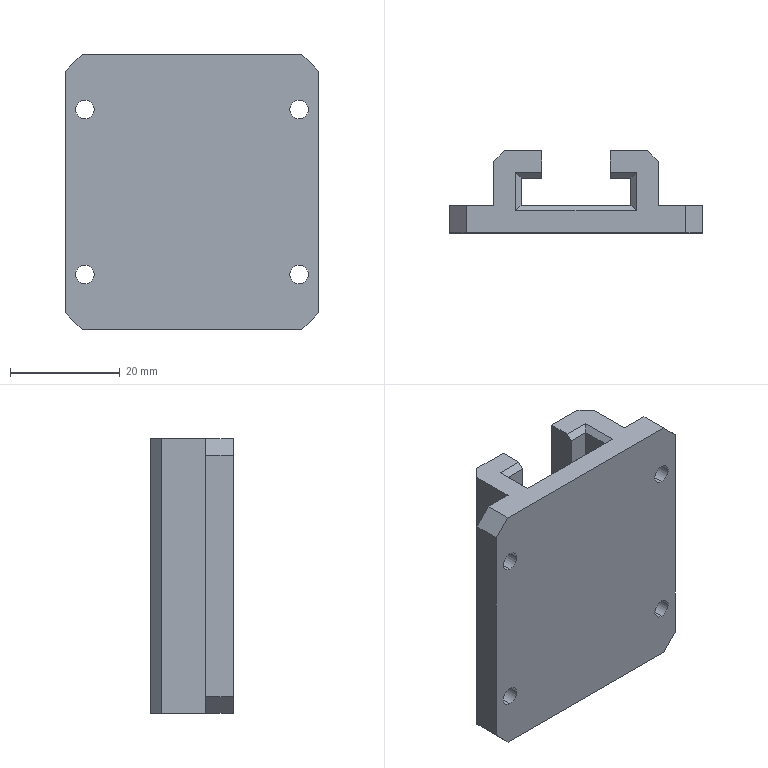Part | SolidWorks | features Chamfer 4, Extrusion 1, HoleWzd 1, ICE 1 | 1 solid | 42 faces | box 46 x 15 x 50 mm | volume 17863 mm3 | plane 34 | cylinder 8 | commonest cylinder face diameters 3.4 x8
STEP:
#1=CARTESIAN_POINT('',(-19.5,0.,8.3));
#2=VERTEX_POINT('',#1);
#3=CARTESIAN_POINT('',(-19.5,0.,11.7));
#4=VERTEX_POINT('',#3);
#5=CARTESIAN_POINT('',(-19.5,0.,10.));
#6=DIRECTION('',(0.,1.,0.));
#7=DIRECTION('',(0.,0.,1.));
#8=AXIS2_PLACEMENT_3D('',#5,#6,#7);
#9=CIRCLE('',#8,1.7);
#10=EDGE_CURVE('',#2,#4,#9,.T.);
#11=ORIENTED_EDGE('',*,*,#10,.F.);
#12=CARTESIAN_POINT('',(-19.5,5.,8.3));
#13=VERTEX_POINT('',#12);
#14=CARTESIAN_POINT('',(-19.5,5.,8.3));
#15=DIRECTION('',(0.,1.,0.));
#16=VECTOR('',#15,1000.);
#17=LINE('',#14,#16);
#18=EDGE_CURVE('',#2,#13,#17,.T.);
#19=ORIENTED_EDGE('',*,*,#18,.T.);
#20=CARTESIAN_POINT('',(-19.5,5.,11.7));
#21=VERTEX_POINT('',#20);
#22=CARTESIAN_POINT('',(-19.5,5.,10.));
#23=DIRECTION('',(0.,1.,0.));
#24=DIRECTION('',(0.,0.,1.));
#25=AXIS2_PLACEMENT_3D('',#22,#23,#24);
#26=CIRCLE('',#25,1.7);
#27=EDGE_CURVE('',#13,#21,#26,.T.);
#28=ORIENTED_EDGE('',*,*,#27,.T.);
#29=CARTESIAN_POINT('',(-19.5,5.,11.7));
#30=DIRECTION('',(0.,1.,0.));
#31=VECTOR('',#30,1000.);
#32=LINE('',#29,#31);
#33=EDGE_CURVE('',#4,#21,#32,.T.);
#34=ORIENTED_EDGE('',*,*,#33,.F.);
#35=EDGE_LOOP('',(#11,#19,#28,#34));
#36=FACE_OUTER_BOUND('',#35,.T.);
#37=CARTESIAN_POINT('',(-19.5,5.,10.));
#38=DIRECTION('',(0.,1.,0.));
#39=DIRECTION('',(0.,0.,1.));
#40=AXIS2_PLACEMENT_3D('',#37,#38,#39);
#41=CYLINDRICAL_SURFACE('',#40,1.7);
#42=ADVANCED_FACE('',(#36),#41,.F.);
#43=CARTESIAN_POINT('',(-19.5,0.,38.3));
#44=VERTEX_POINT('',#43);
#45=CARTESIAN_POINT('',(-19.5,0.,41.7));
#46=VERTEX_POINT('',#45);
#47=CARTESIAN_POINT('',(-19.5,0.,40.));
#48=DIRECTION('',(0.,1.,0.));
#49=DIRECTION('',(0.,0.,1.));
#50=AXIS2_PLACEMENT_3D('',#47,#48,#49);
#51=CIRCLE('',#50,1.7);
#52=EDGE_CURVE('',#44,#46,#51,.T.);
#53=ORIENTED_EDGE('',*,*,#52,.F.);
#54=CARTESIAN_POINT('',(-19.5,5.,38.3));
#55=VERTEX_POINT('',#54);
#56=CARTESIAN_POINT('',(-19.5,5.,38.3));
#57=DIRECTION('',(0.,1.,0.));
#58=VECTOR('',#57,1000.);
#59=LINE('',#56,#58);
#60=EDGE_CURVE('',#44,#55,#59,.T.);
#61=ORIENTED_EDGE('',*,*,#60,.T.);
#62=CARTESIAN_POINT('',(-19.5,5.,41.7));
#63=VERTEX_POINT('',#62);
#64=CARTESIAN_POINT('',(-19.5,5.,40.));
#65=DIRECTION('',(0.,1.,0.));
#66=DIRECTION('',(0.,0.,1.));
#67=AXIS2_PLACEMENT_3D('',#64,#65,#66);
#68=CIRCLE('',#67,1.7);
#69=EDGE_CURVE('',#55,#63,#68,.T.);
#70=ORIENTED_EDGE('',*,*,#69,.T.);
#71=CARTESIAN_POINT('',(-19.5,5.,41.7));
#72=DIRECTION('',(0.,1.,0.));
#73=VECTOR('',#72,1000.);
#74=LINE('',#71,#73);
#75=EDGE_CURVE('',#46,#63,#74,.T.);
#76=ORIENTED_EDGE('',*,*,#75,.F.);
#77=EDGE_LOOP('',(#53,#61,#70,#76));
#78=FACE_OUTER_BOUND('',#77,.T.);
#79=CARTESIAN_POINT('',(-19.5,5.,40.));
#80=DIRECTION('',(0.,1.,0.));
#81=DIRECTION('',(0.,0.,1.));
#82=AXIS2_PLACEMENT_3D('',#79,#80,#81);
#83=CYLINDRICAL_SURFACE('',#82,1.7);
#84=ADVANCED_FACE('',(#78),#83,.F.);
#85=CARTESIAN_POINT('',(19.5,0.,38.3));
#86=VERTEX_POINT('',#85);
#87=CARTESIAN_POINT('',(19.5,0.,41.7));
#88=VERTEX_POINT('',#87);
#89=CARTESIAN_POINT('',(19.5,0.,40.));
#90=DIRECTION('',(0.,1.,0.));
#91=DIRECTION('',(0.,0.,1.));
#92=AXIS2_PLACEMENT_3D('',#89,#90,#91);
#93=CIRCLE('',#92,1.7);
#94=EDGE_CURVE('',#86,#88,#93,.T.);
#95=ORIENTED_EDGE('',*,*,#94,.F.);
#96=CARTESIAN_POINT('',(19.5,5.,38.3));
#97=VERTEX_POINT('',#96);
#98=CARTESIAN_POINT('',(19.5,5.,38.3));
#99=DIRECTION('',(0.,1.,0.));
#100=VECTOR('',#99,1000.);
#101=LINE('',#98,#100);
#102=EDGE_CURVE('',#86,#97,#101,.T.);
#103=ORIENTED_EDGE('',*,*,#102,.T.);
#104=CARTESIAN_POINT('',(19.5,5.,41.7));
#105=VERTEX_POINT('',#104);
#106=CARTESIAN_POINT('',(19.5,5.,40.));
#107=DIRECTION('',(0.,1.,0.));
#108=DIRECTION('',(0.,0.,1.));
#109=AXIS2_PLACEMENT_3D('',#106,#107,#108);
#110=CIRCLE('',#109,1.7);
#111=EDGE_CURVE('',#97,#105,#110,.T.);
#112=ORIENTED_EDGE('',*,*,#111,.T.);
#113=CARTESIAN_POINT('',(19.5,5.,41.7));
#114=DIRECTION('',(0.,1.,0.));
#115=VECTOR('',#114,1000.);
#116=LINE('',#113,#115);
#117=EDGE_CURVE('',#88,#105,#116,.T.);
#118=ORIENTED_EDGE('',*,*,#117,.F.);
#119=EDGE_LOOP('',(#95,#103,#112,#118));
#120=FACE_OUTER_BOUND('',#119,.T.);
#121=CARTESIAN_POINT('',(19.5,5.,40.));
#122=DIRECTION('',(0.,1.,0.));
#123=DIRECTION('',(0.,0.,1.));
#124=AXIS2_PLACEMENT_3D('',#121,#122,#123);
#125=CYLINDRICAL_SURFACE('',#124,1.7);
#126=ADVANCED_FACE('',(#120),#125,.F.);
#127=CARTESIAN_POINT('',(19.5,0.,8.3));
#128=VERTEX_POINT('',#127);
#129=CARTESIAN_POINT('',(19.5,0.,11.7));
#130=VERTEX_POINT('',#129);
#131=CARTESIAN_POINT('',(19.5,0.,10.));
#132=DIRECTION('',(0.,1.,0.));
#133=DIRECTION('',(0.,0.,1.));
#134=AXIS2_PLACEMENT_3D('',#131,#132,#133);
#135=CIRCLE('',#134,1.7);
#136=EDGE_CURVE('',#128,#130,#135,.T.);
#137=ORIENTED_EDGE('',*,*,#136,.F.);
#138=CARTESIAN_POINT('',(19.5,5.,8.3));
#139=VERTEX_POINT('',#138);
#140=CARTESIAN_POINT('',(19.5,5.,8.3));
#141=DIRECTION('',(0.,1.,0.));
#142=VECTOR('',#141,1000.);
#143=LINE('',#140,#142);
#144=EDGE_CURVE('',#128,#139,#143,.T.);
#145=ORIENTED_EDGE('',*,*,#144,.T.);
#146=CARTESIAN_POINT('',(19.5,5.,11.7));
#147=VERTEX_POINT('',#146);
#148=CARTESIAN_POINT('',(19.5,5.,10.));
#149=DIRECTION('',(0.,1.,0.));
#150=DIRECTION('',(0.,0.,1.));
#151=AXIS2_PLACEMENT_3D('',#148,#149,#150);
#152=CIRCLE('',#151,1.7);
#153=EDGE_CURVE('',#139,#147,#152,.T.);
#154=ORIENTED_EDGE('',*,*,#153,.T.);
#155=CARTESIAN_POINT('',(19.5,5.,11.7));
#156=DIRECTION('',(0.,1.,0.));
#157=VECTOR('',#156,1000.);
#158=LINE('',#155,#157);
#159=EDGE_CURVE('',#130,#147,#158,.T.);
#160=ORIENTED_EDGE('',*,*,#159,.F.);
#161=EDGE_LOOP('',(#137,#145,#154,#160));
#162=FACE_OUTER_BOUND('',#161,.T.);
#163=CARTESIAN_POINT('',(19.5,5.,10.));
#164=DIRECTION('',(0.,1.,0.));
#165=DIRECTION('',(0.,0.,1.));
#166=AXIS2_PLACEMENT_3D('',#163,#164,#165);
#167=CYLINDRICAL_SURFACE('',#166,1.7);
#168=ADVANCED_FACE('',(#162),#167,.F.);
#169=CARTESIAN_POINT('',(15.,5.,0.));
#170=VERTEX_POINT('',#169);
#171=CARTESIAN_POINT('',(15.,13.,0.));
#172=VERTEX_POINT('',#171);
#173=CARTESIAN_POINT('',(15.,0.,0.));
#174=DIRECTION('',(0.,1.,0.));
#175=VECTOR('',#174,1000.);
#176=LINE('',#173,#175);
#177=EDGE_CURVE('',#170,#172,#176,.T.);
#178=ORIENTED_EDGE('',*,*,#177,.T.);
#179=CARTESIAN_POINT('',(15.,13.,50.));
#180=VERTEX_POINT('',#179);
#181=CARTESIAN_POINT('',(15.,13.,50.));
#182=DIRECTION('',(0.,0.,1.));
#183=VECTOR('',#182,1000.);
#184=LINE('',#181,#183);
#185=EDGE_CURVE('',#172,#180,#184,.T.);
#186=ORIENTED_EDGE('',*,*,#185,.T.);
#187=CARTESIAN_POINT('',(15.,5.,50.));
#188=VERTEX_POINT('',#187);
#189=CARTESIAN_POINT('',(15.,0.,50.));
#190=DIRECTION('',(0.,1.,0.));
#191=VECTOR('',#190,1000.);
#192=LINE('',#189,#191);
#193=EDGE_CURVE('',#188,#180,#192,.T.);
#194=ORIENTED_EDGE('',*,*,#193,.F.);
#195=CARTESIAN_POINT('',(15.,5.,-9.434));
#196=DIRECTION('',(0.,0.,1.));
#197=VECTOR('',#196,1000.);
#198=LINE('',#195,#197);
#199=EDGE_CURVE('',#170,#188,#198,.T.);
#200=ORIENTED_EDGE('',*,*,#199,.F.);
#201=EDGE_LOOP('',(#178,#186,#194,#200));
#202=FACE_OUTER_BOUND('',#201,.T.);
#203=CARTESIAN_POINT('',(15.,0.,50.));
#204=DIRECTION('',(-1.,0.,0.));
#205=DIRECTION('',(0.,0.,1.));
#206=AXIS2_PLACEMENT_3D('',#203,#204,#205);
#207=PLANE('',#206);
#208=ADVANCED_FACE('',(#202),#207,.F.);
#209=CARTESIAN_POINT('',(-15.,13.,50.));
#210=VERTEX_POINT('',#209);
#211=CARTESIAN_POINT('',(-15.,5.,50.));
#212=VERTEX_POINT('',#211);
#213=CARTESIAN_POINT('',(-15.,0.,50.));
#214=DIRECTION('',(0.,-1.,0.));
#215=VECTOR('',#214,1000.);
#216=LINE('',#213,#215);
#217=EDGE_CURVE('',#210,#212,#216,.T.);
#218=ORIENTED_EDGE('',*,*,#217,.F.);
#219=CARTESIAN_POINT('',(-15.,13.,0.));
#220=VERTEX_POINT('',#219);
#221=CARTESIAN_POINT('',(-15.,13.,50.));
#222=DIRECTION('',(0.,0.,-1.));
#223=VECTOR('',#222,1000.);
#224=LINE('',#221,#223);
#225=EDGE_CURVE('',#210,#220,#224,.T.);
#226=ORIENTED_EDGE('',*,*,#225,.T.);
#227=CARTESIAN_POINT('',(-15.,5.,0.));
#228=VERTEX_POINT('',#227);
#229=CARTESIAN_POINT('',(-15.,0.,0.));
#230=DIRECTION('',(0.,-1.,0.));
#231=VECTOR('',#230,1000.);
#232=LINE('',#229,#231);
#233=EDGE_CURVE('',#220,#228,#232,.T.);
#234=ORIENTED_EDGE('',*,*,#233,.T.);
#235=CARTESIAN_POINT('',(-15.,5.,-9.434));
#236=DIRECTION('',(0.,0.,1.));
#237=VECTOR('',#236,1000.);
#238=LINE('',#235,#237);
#239=EDGE_CURVE('',#228,#212,#238,.T.);
#240=ORIENTED_EDGE('',*,*,#239,.T.);
#241=EDGE_LOOP('',(#218,#226,#234,#240));
#242=FACE_OUTER_BOUND('',#241,.T.);
#243=CARTESIAN_POINT('',(-15.,0.,50.));
#244=DIRECTION('',(1.,0.,0.));
#245=DIRECTION('',(0.,0.,-1.));
#246=AXIS2_PLACEMENT_3D('',#243,#244,#245);
#247=PLANE('',#246);
#248=ADVANCED_FACE('',(#242),#247,.F.);
#249=CARTESIAN_POINT('',(-19.5,0.,10.));
#250=DIRECTION('',(0.,1.,0.));
#251=DIRECTION('',(0.,0.,1.));
#252=AXIS2_PLACEMENT_3D('',#249,#250,#251);
#253=CIRCLE('',#252,1.7);
#254=EDGE_CURVE('',#4,#2,#253,.T.);
#255=ORIENTED_EDGE('',*,*,#254,.T.);
#256=ORIENTED_EDGE('',*,*,#10,.T.);
#257=EDGE_LOOP('',(#255,#256));
#258=FACE_BOUND('',#257,.T.);
#259=CARTESIAN_POINT('',(-19.5,0.,40.));
#260=DIRECTION('',(0.,1.,0.));
#261=DIRECTION('',(0.,0.,1.));
#262=AXIS2_PLACEMENT_3D('',#259,#260,#261);
#263=CIRCLE('',#262,1.7);
#264=EDGE_CURVE('',#46,#44,#263,.T.);
#265=ORIENTED_EDGE('',*,*,#264,.T.);
#266=ORIENTED_EDGE('',*,*,#52,.T.);
#267=EDGE_LOOP('',(#265,#266));
#268=FACE_BOUND('',#267,.T.);
#269=CARTESIAN_POINT('',(19.5,0.,40.));
#270=DIRECTION('',(0.,1.,0.));
#271=DIRECTION('',(0.,0.,1.));
#272=AXIS2_PLACEMENT_3D('',#269,#270,#271);
#273=CIRCLE('',#272,1.7);
#274=EDGE_CURVE('',#88,#86,#273,.T.);
#275=ORIENTED_EDGE('',*,*,#274,.T.);
#276=ORIENTED_EDGE('',*,*,#94,.T.);
#277=EDGE_LOOP('',(#275,#276));
#278=FACE_BOUND('',#277,.T.);
#279=CARTESIAN_POINT('',(19.5,0.,10.));
#280=DIRECTION('',(0.,1.,0.));
#281=DIRECTION('',(0.,0.,1.));
#282=AXIS2_PLACEMENT_3D('',#279,#280,#281);
#283=CIRCLE('',#282,1.7);
#284=EDGE_CURVE('',#130,#128,#283,.T.);
#285=ORIENTED_EDGE('',*,*,#284,.T.);
#286=ORIENTED_EDGE('',*,*,#136,.T.);
#287=EDGE_LOOP('',(#285,#286));
#288=FACE_BOUND('',#287,.T.);
#289=CARTESIAN_POINT('',(-23.,0.,3.));
#290=VERTEX_POINT('',#289);
#291=CARTESIAN_POINT('',(-23.,0.,47.));
#292=VERTEX_POINT('',#291);
#293=CARTESIAN_POINT('',(-23.,0.,-9.434));
#294=DIRECTION('',(0.,0.,1.));
#295=VECTOR('',#294,1000.);
#296=LINE('',#293,#295);
#297=EDGE_CURVE('',#290,#292,#296,.T.);
#298=ORIENTED_EDGE('',*,*,#297,.F.);
#299=CARTESIAN_POINT('',(-20.,0.,0.));
#300=VERTEX_POINT('',#299);
#301=CARTESIAN_POINT('',(-23.,0.,3.));
#302=DIRECTION('',(0.7071,0.,-0.7071));
#303=VECTOR('',#302,1000.);
#304=LINE('',#301,#303);
#305=EDGE_CURVE('',#290,#300,#304,.T.);
#306=ORIENTED_EDGE('',*,*,#305,.T.);
#307=CARTESIAN_POINT('',(20.,0.,0.));
#308=VERTEX_POINT('',#307);
#309=CARTESIAN_POINT('',(15.,0.,0.));
#310=DIRECTION('',(1.,0.,0.));
#311=VECTOR('',#310,1000.);
#312=LINE('',#309,#311);
#313=EDGE_CURVE('',#300,#308,#312,.T.);
#314=ORIENTED_EDGE('',*,*,#313,.T.);
#315=CARTESIAN_POINT('',(23.,0.,3.));
#316=VERTEX_POINT('',#315);
#317=CARTESIAN_POINT('',(23.,0.,3.));
#318=DIRECTION('',(0.7071,0.,0.7071));
#319=VECTOR('',#318,1000.);
#320=LINE('',#317,#319);
#321=EDGE_CURVE('',#308,#316,#320,.T.);
#322=ORIENTED_EDGE('',*,*,#321,.T.);
#323=CARTESIAN_POINT('',(23.,0.,47.));
#324=VERTEX_POINT('',#323);
#325=CARTESIAN_POINT('',(23.,0.,-9.434));
#326=DIRECTION('',(0.,0.,1.));
#327=VECTOR('',#326,1000.);
#328=LINE('',#325,#327);
#329=EDGE_CURVE('',#316,#324,#328,.T.);
#330=ORIENTED_EDGE('',*,*,#329,.T.);
#331=CARTESIAN_POINT('',(20.,0.,50.));
#332=VERTEX_POINT('',#331);
#333=CARTESIAN_POINT('',(20.,0.,50.));
#334=DIRECTION('',(-0.7071,0.,0.7071));
#335=VECTOR('',#334,1000.);
#336=LINE('',#333,#335);
#337=EDGE_CURVE('',#324,#332,#336,.T.);
#338=ORIENTED_EDGE('',*,*,#337,.T.);
#339=CARTESIAN_POINT('',(-20.,0.,50.));
#340=VERTEX_POINT('',#339);
#341=CARTESIAN_POINT('',(15.,0.,50.));
#342=DIRECTION('',(1.,0.,0.));
#343=VECTOR('',#342,1000.);
#344=LINE('',#341,#343);
#345=EDGE_CURVE('',#340,#332,#344,.T.);
#346=ORIENTED_EDGE('',*,*,#345,.F.);
#347=CARTESIAN_POINT('',(-20.,0.,50.));
#348=DIRECTION('',(-0.7071,0.,-0.7071));
#349=VECTOR('',#348,1000.);
#350=LINE('',#347,#349);
#351=EDGE_CURVE('',#340,#292,#350,.T.);
#352=ORIENTED_EDGE('',*,*,#351,.T.);
#353=EDGE_LOOP('',(#298,#306,#314,#322,#330,#338,#346,#352));
#354=FACE_OUTER_BOUND('',#353,.T.);
#355=CARTESIAN_POINT('',(15.,0.,50.));
#356=DIRECTION('',(0.,1.,0.));
#357=DIRECTION('',(0.,0.,1.));
#358=AXIS2_PLACEMENT_3D('',#355,#356,#357);
#359=PLANE('',#358);
#360=ADVANCED_FACE('',(#258,#268,#278,#288,#354),#359,.F.);
#361=CARTESIAN_POINT('',(13.,15.,50.));
#362=VERTEX_POINT('',#361);
#363=CARTESIAN_POINT('',(6.25,15.,50.));
#364=VERTEX_POINT('',#363);
#365=CARTESIAN_POINT('',(15.,15.,50.));
#366=DIRECTION('',(-1.,0.,0.));
#367=VECTOR('',#366,1000.);
#368=LINE('',#365,#367);
#369=EDGE_CURVE('',#362,#364,#368,.T.);
#370=ORIENTED_EDGE('',*,*,#369,.F.);
#371=CARTESIAN_POINT('',(13.,15.,0.));
#372=VERTEX_POINT('',#371);
#373=CARTESIAN_POINT('',(13.,15.,50.));
#374=DIRECTION('',(0.,0.,-1.));
#375=VECTOR('',#374,1000.);
#376=LINE('',#373,#375);
#377=EDGE_CURVE('',#362,#372,#376,.T.);
#378=ORIENTED_EDGE('',*,*,#377,.T.);
#379=CARTESIAN_POINT('',(6.25,15.,0.));
#380=VERTEX_POINT('',#379);
#381=CARTESIAN_POINT('',(15.,15.,0.));
#382=DIRECTION('',(-1.,0.,0.));
#383=VECTOR('',#382,1000.);
#384=LINE('',#381,#383);
#385=EDGE_CURVE('',#372,#380,#384,.T.);
#386=ORIENTED_EDGE('',*,*,#385,.T.);
#387=CARTESIAN_POINT('',(6.25,15.,50.));
#388=DIRECTION('',(0.,0.,-1.));
#389=VECTOR('',#388,1000.);
#390=LINE('',#387,#389);
#391=EDGE_CURVE('',#364,#380,#390,.T.);
#392=ORIENTED_EDGE('',*,*,#391,.F.);
#393=EDGE_LOOP('',(#370,#378,#386,#392));
#394=FACE_OUTER_BOUND('',#393,.T.);
#395=CARTESIAN_POINT('',(15.,15.,50.));
#396=DIRECTION('',(0.,-1.,0.));
#397=DIRECTION('',(0.,0.,-1.));
#398=AXIS2_PLACEMENT_3D('',#395,#396,#397);
#399=PLANE('',#398);
#400=ADVANCED_FACE('',(#394),#399,.F.);
#401=CARTESIAN_POINT('',(6.25,11.,0.));
#402=VERTEX_POINT('',#401);
#403=CARTESIAN_POINT('',(6.25,15.,0.));
#404=DIRECTION('',(0.,-1.,0.));
#405=VECTOR('',#404,1000.);
#406=LINE('',#403,#405);
#407=EDGE_CURVE('',#380,#402,#406,.T.);
#408=ORIENTED_EDGE('',*,*,#407,.T.);
#409=CARTESIAN_POINT('',(6.25,10.,1.));
#410=VERTEX_POINT('',#409);
#411=CARTESIAN_POINT('',(6.25,10.,1.));
#412=DIRECTION('',(0.,-0.7071,0.7071));
#413=VECTOR('',#412,1000.);
#414=LINE('',#411,#413);
#415=EDGE_CURVE('',#402,#410,#414,.T.);
#416=ORIENTED_EDGE('',*,*,#415,.T.);
#417=CARTESIAN_POINT('',(6.25,10.,49.));
#418=VERTEX_POINT('',#417);
#419=CARTESIAN_POINT('',(6.25,10.,50.));
#420=DIRECTION('',(0.,0.,-1.));
#421=VECTOR('',#420,1000.);
#422=LINE('',#419,#421);
#423=EDGE_CURVE('',#418,#410,#422,.T.);
#424=ORIENTED_EDGE('',*,*,#423,.F.);
#425=CARTESIAN_POINT('',(6.25,11.,50.));
#426=VERTEX_POINT('',#425);
#427=CARTESIAN_POINT('',(6.25,11.,50.));
#428=DIRECTION('',(0.,0.7071,0.7071));
#429=VECTOR('',#428,1000.);
#430=LINE('',#427,#429);
#431=EDGE_CURVE('',#418,#426,#430,.T.);
#432=ORIENTED_EDGE('',*,*,#431,.T.);
#433=CARTESIAN_POINT('',(6.25,15.,50.));
#434=DIRECTION('',(0.,-1.,0.));
#435=VECTOR('',#434,1000.);
#436=LINE('',#433,#435);
#437=EDGE_CURVE('',#364,#426,#436,.T.);
#438=ORIENTED_EDGE('',*,*,#437,.F.);
#439=ORIENTED_EDGE('',*,*,#391,.T.);
#440=EDGE_LOOP('',(#408,#416,#424,#432,#438,#439));
#441=FACE_OUTER_BOUND('',#440,.T.);
#442=CARTESIAN_POINT('',(6.25,15.,50.));
#443=DIRECTION('',(1.,0.,0.));
#444=DIRECTION('',(0.,1.,0.));
#445=AXIS2_PLACEMENT_3D('',#442,#443,#444);
#446=PLANE('',#445);
#447=ADVANCED_FACE('',(#441),#446,.F.);
#448=ORIENTED_EDGE('',*,*,#423,.T.);
#449=CARTESIAN_POINT('',(10.,10.,1.));
#450=VERTEX_POINT('',#449);
#451=CARTESIAN_POINT('',(10.,10.,1.));
#452=DIRECTION('',(1.,0.,0.));
#453=VECTOR('',#452,1000.);
#454=LINE('',#451,#453);
#455=EDGE_CURVE('',#410,#450,#454,.T.);
#456=ORIENTED_EDGE('',*,*,#455,.T.);
#457=CARTESIAN_POINT('',(10.,10.,49.));
#458=VERTEX_POINT('',#457);
#459=CARTESIAN_POINT('',(10.,10.,50.));
#460=DIRECTION('',(0.,0.,-1.));
#461=VECTOR('',#460,1000.);
#462=LINE('',#459,#461);
#463=EDGE_CURVE('',#458,#450,#462,.T.);
#464=ORIENTED_EDGE('',*,*,#463,.F.);
#465=CARTESIAN_POINT('',(6.25,10.,49.));
#466=DIRECTION('',(-1.,0.,0.));
#467=VECTOR('',#466,1000.);
#468=LINE('',#465,#467);
#469=EDGE_CURVE('',#458,#418,#468,.T.);
#470=ORIENTED_EDGE('',*,*,#469,.T.);
#471=EDGE_LOOP('',(#448,#456,#464,#470));
#472=FACE_OUTER_BOUND('',#471,.T.);
#473=CARTESIAN_POINT('',(6.25,10.,50.));
#474=DIRECTION('',(0.,1.,0.));
#475=DIRECTION('',(0.,0.,1.));
#476=AXIS2_PLACEMENT_3D('',#473,#474,#475);
#477=PLANE('',#476);
#478=ADVANCED_FACE('',(#472),#477,.F.);
#479=ORIENTED_EDGE('',*,*,#463,.T.);
#480=CARTESIAN_POINT('',(10.,5.,1.));
#481=VERTEX_POINT('',#480);
#482=CARTESIAN_POINT('',(10.,5.,1.));
#483=DIRECTION('',(0.,-1.,0.));
#484=VECTOR('',#483,1000.);
#485=LINE('',#482,#484);
#486=EDGE_CURVE('',#450,#481,#485,.T.);
#487=ORIENTED_EDGE('',*,*,#486,.T.);
#488=CARTESIAN_POINT('',(10.,5.,49.));
#489=VERTEX_POINT('',#488);
#490=CARTESIAN_POINT('',(10.,5.,50.));
#491=DIRECTION('',(0.,0.,-1.));
#492=VECTOR('',#491,1000.);
#493=LINE('',#490,#492);
#494=EDGE_CURVE('',#489,#481,#493,.T.);
#495=ORIENTED_EDGE('',*,*,#494,.F.);
#496=CARTESIAN_POINT('',(10.,10.,49.));
#497=DIRECTION('',(0.,1.,0.));
#498=VECTOR('',#497,1000.);
#499=LINE('',#496,#498);
#500=EDGE_CURVE('',#489,#458,#499,.T.);
#501=ORIENTED_EDGE('',*,*,#500,.T.);
#502=EDGE_LOOP('',(#479,#487,#495,#501));
#503=FACE_OUTER_BOUND('',#502,.T.);
#504=CARTESIAN_POINT('',(10.,10.,50.));
#505=DIRECTION('',(1.,0.,0.));
#506=DIRECTION('',(0.,0.,-1.));
#507=AXIS2_PLACEMENT_3D('',#504,#505,#506);
#508=PLANE('',#507);
#509=ADVANCED_FACE('',(#503),#508,.F.);
#510=ORIENTED_EDGE('',*,*,#494,.T.);
#511=CARTESIAN_POINT('',(-10.,5.,1.));
#512=VERTEX_POINT('',#511);
#513=CARTESIAN_POINT('',(-10.,5.,1.));
#514=DIRECTION('',(-1.,0.,0.));
#515=VECTOR('',#514,1000.);
#516=LINE('',#513,#515);
#517=EDGE_CURVE('',#481,#512,#516,.T.);
#518=ORIENTED_EDGE('',*,*,#517,.T.);
#519=CARTESIAN_POINT('',(-10.,5.,49.));
#520=VERTEX_POINT('',#519);
#521=CARTESIAN_POINT('',(-10.,5.,50.));
#522=DIRECTION('',(0.,0.,-1.));
#523=VECTOR('',#522,1000.);
#524=LINE('',#521,#523);
#525=EDGE_CURVE('',#520,#512,#524,.T.);
#526=ORIENTED_EDGE('',*,*,#525,.F.);
#527=CARTESIAN_POINT('',(-10.,5.,49.));
#528=DIRECTION('',(1.,0.,0.));
#529=VECTOR('',#528,1000.);
#530=LINE('',#527,#529);
#531=EDGE_CURVE('',#520,#489,#530,.T.);
#532=ORIENTED_EDGE('',*,*,#531,.T.);
#533=EDGE_LOOP('',(#510,#518,#526,#532));
#534=FACE_OUTER_BOUND('',#533,.T.);
#535=CARTESIAN_POINT('',(-10.,5.,50.));
#536=DIRECTION('',(0.,-1.,0.));
#537=DIRECTION('',(0.,0.,-1.));
#538=AXIS2_PLACEMENT_3D('',#535,#536,#537);
#539=PLANE('',#538);
#540=ADVANCED_FACE('',(#534),#539,.F.);
#541=ORIENTED_EDGE('',*,*,#525,.T.);
#542=CARTESIAN_POINT('',(-10.,10.,1.));
#543=VERTEX_POINT('',#542);
#544=CARTESIAN_POINT('',(-10.,10.,1.));
#545=DIRECTION('',(0.,1.,0.));
#546=VECTOR('',#545,1000.);
#547=LINE('',#544,#546);
#548=EDGE_CURVE('',#512,#543,#547,.T.);
#549=ORIENTED_EDGE('',*,*,#548,.T.);
#550=CARTESIAN_POINT('',(-10.,10.,49.));
#551=VERTEX_POINT('',#550);
#552=CARTESIAN_POINT('',(-10.,10.,50.));
#553=DIRECTION('',(0.,0.,-1.));
#554=VECTOR('',#553,1000.);
#555=LINE('',#552,#554);
#556=EDGE_CURVE('',#551,#543,#555,.T.);
#557=ORIENTED_EDGE('',*,*,#556,.F.);
#558=CARTESIAN_POINT('',(-10.,10.,49.));
#559=DIRECTION('',(0.,-1.,0.));
#560=VECTOR('',#559,1000.);
#561=LINE('',#558,#560);
#562=EDGE_CURVE('',#551,#520,#561,.T.);
#563=ORIENTED_EDGE('',*,*,#562,.T.);
#564=EDGE_LOOP('',(#541,#549,#557,#563));
#565=FACE_OUTER_BOUND('',#564,.T.);
#566=CARTESIAN_POINT('',(-10.,10.,50.));
#567=DIRECTION('',(-1.,0.,0.));
#568=DIRECTION('',(0.,0.,1.));
#569=AXIS2_PLACEMENT_3D('',#566,#567,#568);
#570=PLANE('',#569);
#571=ADVANCED_FACE('',(#565),#570,.F.);
#572=ORIENTED_EDGE('',*,*,#556,.T.);
#573=CARTESIAN_POINT('',(-6.25,10.,1.));
#574=VERTEX_POINT('',#573);
#575=CARTESIAN_POINT('',(-6.25,10.,1.));
#576=DIRECTION('',(1.,0.,0.));
#577=VECTOR('',#576,1000.);
#578=LINE('',#575,#577);
#579=EDGE_CURVE('',#543,#574,#578,.T.);
#580=ORIENTED_EDGE('',*,*,#579,.T.);
#581=CARTESIAN_POINT('',(-6.25,10.,49.));
#582=VERTEX_POINT('',#581);
#583=CARTESIAN_POINT('',(-6.25,10.,50.));
#584=DIRECTION('',(0.,0.,-1.));
#585=VECTOR('',#584,1000.);
#586=LINE('',#583,#585);
#587=EDGE_CURVE('',#582,#574,#586,.T.);
#588=ORIENTED_EDGE('',*,*,#587,.F.);
#589=CARTESIAN_POINT('',(-6.25,10.,49.));
#590=DIRECTION('',(-1.,0.,0.));
#591=VECTOR('',#590,1000.);
#592=LINE('',#589,#591);
#593=EDGE_CURVE('',#582,#551,#592,.T.);
#594=ORIENTED_EDGE('',*,*,#593,.T.);
#595=EDGE_LOOP('',(#572,#580,#588,#594));
#596=FACE_OUTER_BOUND('',#595,.T.);
#597=CARTESIAN_POINT('',(-6.25,10.,50.));
#598=DIRECTION('',(0.,1.,0.));
#599=DIRECTION('',(0.,0.,1.));
#600=AXIS2_PLACEMENT_3D('',#597,#598,#599);
#601=PLANE('',#600);
#602=ADVANCED_FACE('',(#596),#601,.F.);
#603=ORIENTED_EDGE('',*,*,#587,.T.);
#604=CARTESIAN_POINT('',(-6.25,11.,0.));
#605=VERTEX_POINT('',#604);
#606=CARTESIAN_POINT('',(-6.25,10.,1.));
#607=DIRECTION('',(0.,0.7071,-0.7071));
#608=VECTOR('',#607,1000.);
#609=LINE('',#606,#608);
#610=EDGE_CURVE('',#574,#605,#609,.T.);
#611=ORIENTED_EDGE('',*,*,#610,.T.);
#612=CARTESIAN_POINT('',(-6.25,15.,0.));
#613=VERTEX_POINT('',#612);
#614=CARTESIAN_POINT('',(-6.25,15.,0.));
#615=DIRECTION('',(0.,1.,0.));
#616=VECTOR('',#615,1000.);
#617=LINE('',#614,#616);
#618=EDGE_CURVE('',#605,#613,#617,.T.);
#619=ORIENTED_EDGE('',*,*,#618,.T.);
#620=CARTESIAN_POINT('',(-6.25,15.,50.));
#621=VERTEX_POINT('',#620);
#622=CARTESIAN_POINT('',(-6.25,15.,50.));
#623=DIRECTION('',(0.,0.,-1.));
#624=VECTOR('',#623,1000.);
#625=LINE('',#622,#624);
#626=EDGE_CURVE('',#621,#613,#625,.T.);
#627=ORIENTED_EDGE('',*,*,#626,.F.);
#628=CARTESIAN_POINT('',(-6.25,11.,50.));
#629=VERTEX_POINT('',#628);
#630=CARTESIAN_POINT('',(-6.25,15.,50.));
#631=DIRECTION('',(0.,1.,0.));
#632=VECTOR('',#631,1000.);
#633=LINE('',#630,#632);
#634=EDGE_CURVE('',#629,#621,#633,.T.);
#635=ORIENTED_EDGE('',*,*,#634,.F.);
#636=CARTESIAN_POINT('',(-6.25,11.,50.));
#637=DIRECTION('',(0.,-0.7071,-0.7071));
#638=VECTOR('',#637,1000.);
#639=LINE('',#636,#638);
#640=EDGE_CURVE('',#629,#582,#639,.T.);
#641=ORIENTED_EDGE('',*,*,#640,.T.);
#642=EDGE_LOOP('',(#603,#611,#619,#627,#635,#641));
#643=FACE_OUTER_BOUND('',#642,.T.);
#644=CARTESIAN_POINT('',(-6.25,15.,50.));
#645=DIRECTION('',(-1.,0.,0.));
#646=DIRECTION('',(0.,-1.,0.));
#647=AXIS2_PLACEMENT_3D('',#644,#645,#646);
#648=PLANE('',#647);
#649=ADVANCED_FACE('',(#643),#648,.F.);
#650=CARTESIAN_POINT('',(-13.,15.,0.));
#651=VERTEX_POINT('',#650);
#652=CARTESIAN_POINT('',(-15.,15.,0.));
#653=DIRECTION('',(-1.,0.,0.));
#654=VECTOR('',#653,1000.);
#655=LINE('',#652,#654);
#656=EDGE_CURVE('',#613,#651,#655,.T.);
#657=ORIENTED_EDGE('',*,*,#656,.T.);
#658=CARTESIAN_POINT('',(-13.,15.,50.));
#659=VERTEX_POINT('',#658);
#660=CARTESIAN_POINT('',(-13.,15.,50.));
#661=DIRECTION('',(0.,0.,1.));
#662=VECTOR('',#661,1000.);
#663=LINE('',#660,#662);
#664=EDGE_CURVE('',#651,#659,#663,.T.);
#665=ORIENTED_EDGE('',*,*,#664,.T.);
#666=CARTESIAN_POINT('',(-15.,15.,50.));
#667=DIRECTION('',(-1.,0.,0.));
#668=VECTOR('',#667,1000.);
#669=LINE('',#666,#668);
#670=EDGE_CURVE('',#621,#659,#669,.T.);
#671=ORIENTED_EDGE('',*,*,#670,.F.);
#672=ORIENTED_EDGE('',*,*,#626,.T.);
#673=EDGE_LOOP('',(#657,#665,#671,#672));
#674=FACE_OUTER_BOUND('',#673,.T.);
#675=CARTESIAN_POINT('',(-15.,15.,50.));
#676=DIRECTION('',(0.,-1.,0.));
#677=DIRECTION('',(0.,0.,-1.));
#678=AXIS2_PLACEMENT_3D('',#675,#676,#677);
#679=PLANE('',#678);
#680=ADVANCED_FACE('',(#674),#679,.F.);
#681=ORIENTED_EDGE('',*,*,#670,.T.);
#682=CARTESIAN_POINT('',(-15.,13.,50.));
#683=DIRECTION('',(-0.7071,-0.7071,0.));
#684=VECTOR('',#683,1000.);
#685=LINE('',#682,#684);
#686=EDGE_CURVE('',#659,#210,#685,.T.);
#687=ORIENTED_EDGE('',*,*,#686,.T.);
#688=ORIENTED_EDGE('',*,*,#217,.T.);
#689=CARTESIAN_POINT('',(-20.,5.,50.));
#690=VERTEX_POINT('',#689);
#691=CARTESIAN_POINT('',(-15.,5.,50.));
#692=DIRECTION('',(-1.,0.,0.));
#693=VECTOR('',#692,1000.);
#694=LINE('',#691,#693);
#695=EDGE_CURVE('',#212,#690,#694,.T.);
#696=ORIENTED_EDGE('',*,*,#695,.T.);
#697=CARTESIAN_POINT('',(-20.,0.,50.));
#698=DIRECTION('',(0.,-1.,0.));
#699=VECTOR('',#698,1000.);
#700=LINE('',#697,#699);
#701=EDGE_CURVE('',#690,#340,#700,.T.);
#702=ORIENTED_EDGE('',*,*,#701,.T.);
#703=ORIENTED_EDGE('',*,*,#345,.T.);
#704=CARTESIAN_POINT('',(20.,5.,50.));
#705=VERTEX_POINT('',#704);
#706=CARTESIAN_POINT('',(20.,5.,50.));
#707=DIRECTION('',(0.,1.,0.));
#708=VECTOR('',#707,1000.);
#709=LINE('',#706,#708);
#710=EDGE_CURVE('',#332,#705,#709,.T.);
#711=ORIENTED_EDGE('',*,*,#710,.T.);
#712=CARTESIAN_POINT('',(15.,5.,50.));
#713=DIRECTION('',(-1.,0.,0.));
#714=VECTOR('',#713,1000.);
#715=LINE('',#712,#714);
#716=EDGE_CURVE('',#705,#188,#715,.T.);
#717=ORIENTED_EDGE('',*,*,#716,.T.);
#718=ORIENTED_EDGE('',*,*,#193,.T.);
#719=CARTESIAN_POINT('',(13.,15.,50.));
#720=DIRECTION('',(-0.7071,0.7071,0.));
#721=VECTOR('',#720,1000.);
#722=LINE('',#719,#721);
#723=EDGE_CURVE('',#180,#362,#722,.T.);
#724=ORIENTED_EDGE('',*,*,#723,.T.);
#725=ORIENTED_EDGE('',*,*,#369,.T.);
#726=ORIENTED_EDGE('',*,*,#437,.T.);
#727=CARTESIAN_POINT('',(11.,11.,50.));
#728=VERTEX_POINT('',#727);
#729=CARTESIAN_POINT('',(0.,11.,50.));
#730=DIRECTION('',(1.,0.,0.));
#731=VECTOR('',#730,1000.);
#732=LINE('',#729,#731);
#733=EDGE_CURVE('',#426,#728,#732,.T.);
#734=ORIENTED_EDGE('',*,*,#733,.T.);
#735=CARTESIAN_POINT('',(11.,4.,50.));
#736=VERTEX_POINT('',#735);
#737=CARTESIAN_POINT('',(11.,0.,50.));
#738=DIRECTION('',(0.,-1.,0.));
#739=VECTOR('',#738,1000.);
#740=LINE('',#737,#739);
#741=EDGE_CURVE('',#728,#736,#740,.T.);
#742=ORIENTED_EDGE('',*,*,#741,.T.);
#743=CARTESIAN_POINT('',(-11.,4.,50.));
#744=VERTEX_POINT('',#743);
#745=CARTESIAN_POINT('',(0.,4.,50.));
#746=DIRECTION('',(-1.,0.,0.));
#747=VECTOR('',#746,1000.);
#748=LINE('',#745,#747);
#749=EDGE_CURVE('',#736,#744,#748,.T.);
#750=ORIENTED_EDGE('',*,*,#749,.T.);
#751=CARTESIAN_POINT('',(-11.,11.,50.));
#752=VERTEX_POINT('',#751);
#753=CARTESIAN_POINT('',(-11.,0.,50.));
#754=DIRECTION('',(0.,1.,0.));
#755=VECTOR('',#754,1000.);
#756=LINE('',#753,#755);
#757=EDGE_CURVE('',#744,#752,#756,.T.);
#758=ORIENTED_EDGE('',*,*,#757,.T.);
#759=CARTESIAN_POINT('',(0.,11.,50.));
#760=DIRECTION('',(1.,0.,0.));
#761=VECTOR('',#760,1000.);
#762=LINE('',#759,#761);
#763=EDGE_CURVE('',#752,#629,#762,.T.);
#764=ORIENTED_EDGE('',*,*,#763,.T.);
#765=ORIENTED_EDGE('',*,*,#634,.T.);
#766=EDGE_LOOP('',(#681,#687,#688,#696,#702,#703,#711,#717,#718,#724,#725,#726,#734,#742,#750,#758,#764,#765));
#767=FACE_OUTER_BOUND('',#766,.T.);
#768=CARTESIAN_POINT('',(0.,0.,50.));
#769=DIRECTION('',(0.,0.,-1.));
#770=DIRECTION('',(-1.,0.,0.));
#771=AXIS2_PLACEMENT_3D('',#768,#769,#770);
#772=PLANE('',#771);
#773=ADVANCED_FACE('',(#767),#772,.F.);
#774=ORIENTED_EDGE('',*,*,#233,.F.);
#775=CARTESIAN_POINT('',(-14.,14.,0.));
#776=DIRECTION('',(0.7071,0.7071,0.));
#777=VECTOR('',#776,1000.);
#778=LINE('',#775,#777);
#779=EDGE_CURVE('',#220,#651,#778,.T.);
#780=ORIENTED_EDGE('',*,*,#779,.T.);
#781=ORIENTED_EDGE('',*,*,#656,.F.);
#782=ORIENTED_EDGE('',*,*,#618,.F.);
#783=CARTESIAN_POINT('',(-11.,11.,0.));
#784=VERTEX_POINT('',#783);
#785=CARTESIAN_POINT('',(-10.,11.,0.));
#786=DIRECTION('',(-1.,0.,0.));
#787=VECTOR('',#786,1000.);
#788=LINE('',#785,#787);
#789=EDGE_CURVE('',#605,#784,#788,.T.);
#790=ORIENTED_EDGE('',*,*,#789,.T.);
#791=CARTESIAN_POINT('',(-11.,4.,0.));
#792=VERTEX_POINT('',#791);
#793=CARTESIAN_POINT('',(-11.,5.,0.));
#794=DIRECTION('',(0.,-1.,0.));
#795=VECTOR('',#794,1000.);
#796=LINE('',#793,#795);
#797=EDGE_CURVE('',#784,#792,#796,.T.);
#798=ORIENTED_EDGE('',*,*,#797,.T.);
#799=CARTESIAN_POINT('',(11.,4.,0.));
#800=VERTEX_POINT('',#799);
#801=CARTESIAN_POINT('',(10.,4.,0.));
#802=DIRECTION('',(1.,0.,0.));
#803=VECTOR('',#802,1000.);
#804=LINE('',#801,#803);
#805=EDGE_CURVE('',#792,#800,#804,.T.);
#806=ORIENTED_EDGE('',*,*,#805,.T.);
#807=CARTESIAN_POINT('',(11.,11.,0.));
#808=VERTEX_POINT('',#807);
#809=CARTESIAN_POINT('',(11.,10.,0.));
#810=DIRECTION('',(0.,1.,0.));
#811=VECTOR('',#810,1000.);
#812=LINE('',#809,#811);
#813=EDGE_CURVE('',#800,#808,#812,.T.);
#814=ORIENTED_EDGE('',*,*,#813,.T.);
#815=CARTESIAN_POINT('',(6.25,11.,0.));
#816=DIRECTION('',(-1.,0.,0.));
#817=VECTOR('',#816,1000.);
#818=LINE('',#815,#817);
#819=EDGE_CURVE('',#808,#402,#818,.T.);
#820=ORIENTED_EDGE('',*,*,#819,.T.);
#821=ORIENTED_EDGE('',*,*,#407,.F.);
#822=ORIENTED_EDGE('',*,*,#385,.F.);
#823=CARTESIAN_POINT('',(14.,14.,0.));
#824=DIRECTION('',(0.7071,-0.7071,0.));
#825=VECTOR('',#824,1000.);
#826=LINE('',#823,#825);
#827=EDGE_CURVE('',#372,#172,#826,.T.);
#828=ORIENTED_EDGE('',*,*,#827,.T.);
#829=ORIENTED_EDGE('',*,*,#177,.F.);
#830=CARTESIAN_POINT('',(20.,5.,0.));
#831=VERTEX_POINT('',#830);
#832=CARTESIAN_POINT('',(15.,5.,0.));
#833=DIRECTION('',(-1.,0.,0.));
#834=VECTOR('',#833,1000.);
#835=LINE('',#832,#834);
#836=EDGE_CURVE('',#831,#170,#835,.T.);
#837=ORIENTED_EDGE('',*,*,#836,.F.);
#838=CARTESIAN_POINT('',(20.,0.,0.));
#839=DIRECTION('',(0.,-1.,0.));
#840=VECTOR('',#839,1000.);
#841=LINE('',#838,#840);
#842=EDGE_CURVE('',#831,#308,#841,.T.);
#843=ORIENTED_EDGE('',*,*,#842,.T.);
#844=ORIENTED_EDGE('',*,*,#313,.F.);
#845=CARTESIAN_POINT('',(-20.,5.,0.));
#846=VERTEX_POINT('',#845);
#847=CARTESIAN_POINT('',(-20.,0.,0.));
#848=DIRECTION('',(0.,1.,0.));
#849=VECTOR('',#848,1000.);
#850=LINE('',#847,#849);
#851=EDGE_CURVE('',#300,#846,#850,.T.);
#852=ORIENTED_EDGE('',*,*,#851,.T.);
#853=CARTESIAN_POINT('',(-15.,5.,0.));
#854=DIRECTION('',(-1.,0.,0.));
#855=VECTOR('',#854,1000.);
#856=LINE('',#853,#855);
#857=EDGE_CURVE('',#228,#846,#856,.T.);
#858=ORIENTED_EDGE('',*,*,#857,.F.);
#859=EDGE_LOOP('',(#774,#780,#781,#782,#790,#798,#806,#814,#820,#821,#822,#828,#829,#837,#843,#844,#852,#858));
#860=FACE_OUTER_BOUND('',#859,.T.);
#861=CARTESIAN_POINT('',(0.,0.,0.));
#862=DIRECTION('',(0.,0.,-1.));
#863=DIRECTION('',(-1.,0.,0.));
#864=AXIS2_PLACEMENT_3D('',#861,#862,#863);
#865=PLANE('',#864);
#866=ADVANCED_FACE('',(#860),#865,.T.);
#867=CARTESIAN_POINT('',(-19.5,5.,10.));
#868=DIRECTION('',(0.,1.,0.));
#869=DIRECTION('',(0.,0.,1.));
#870=AXIS2_PLACEMENT_3D('',#867,#868,#869);
#871=CIRCLE('',#870,1.7);
#872=EDGE_CURVE('',#21,#13,#871,.T.);
#873=ORIENTED_EDGE('',*,*,#872,.F.);
#874=ORIENTED_EDGE('',*,*,#27,.F.);
#875=EDGE_LOOP('',(#873,#874));
#876=FACE_BOUND('',#875,.T.);
#877=CARTESIAN_POINT('',(-19.5,5.,40.));
#878=DIRECTION('',(0.,1.,0.));
#879=DIRECTION('',(0.,0.,1.));
#880=AXIS2_PLACEMENT_3D('',#877,#878,#879);
#881=CIRCLE('',#880,1.7);
#882=EDGE_CURVE('',#63,#55,#881,.T.);
#883=ORIENTED_EDGE('',*,*,#882,.F.);
#884=ORIENTED_EDGE('',*,*,#69,.F.);
#885=EDGE_LOOP('',(#883,#884));
#886=FACE_BOUND('',#885,.T.);
#887=ORIENTED_EDGE('',*,*,#857,.T.);
#888=CARTESIAN_POINT('',(-23.,5.,3.));
#889=VERTEX_POINT('',#888);
#890=CARTESIAN_POINT('',(-12.783,5.,-7.217));
#891=DIRECTION('',(-0.7071,0.,0.7071));
#892=VECTOR('',#891,1000.);
#893=LINE('',#890,#892);
#894=EDGE_CURVE('',#846,#889,#893,.T.);
#895=ORIENTED_EDGE('',*,*,#894,.T.);
#896=CARTESIAN_POINT('',(-23.,5.,47.));
#897=VERTEX_POINT('',#896);
#898=CARTESIAN_POINT('',(-23.,5.,-9.434));
#899=DIRECTION('',(0.,0.,1.));
#900=VECTOR('',#899,1000.);
#901=LINE('',#898,#900);
#902=EDGE_CURVE('',#889,#897,#901,.T.);
#903=ORIENTED_EDGE('',*,*,#902,.T.);
#904=CARTESIAN_POINT('',(-47.217,5.,22.783));
#905=DIRECTION('',(0.7071,0.,0.7071));
#906=VECTOR('',#905,1000.);
#907=LINE('',#904,#906);
#908=EDGE_CURVE('',#897,#690,#907,.T.);
#909=ORIENTED_EDGE('',*,*,#908,.T.);
#910=ORIENTED_EDGE('',*,*,#695,.F.);
#911=ORIENTED_EDGE('',*,*,#239,.F.);
#912=EDGE_LOOP('',(#887,#895,#903,#909,#910,#911));
#913=FACE_OUTER_BOUND('',#912,.T.);
#914=CARTESIAN_POINT('',(-15.,5.,-9.434));
#915=DIRECTION('',(0.,1.,0.));
#916=DIRECTION('',(-1.,0.,0.));
#917=AXIS2_PLACEMENT_3D('',#914,#915,#916);
#918=PLANE('',#917);
#919=ADVANCED_FACE('',(#876,#886,#913),#918,.T.);
#920=ORIENTED_EDGE('',*,*,#902,.F.);
#921=CARTESIAN_POINT('',(-23.,0.,3.));
#922=DIRECTION('',(0.,-1.,0.));
#923=VECTOR('',#922,1000.);
#924=LINE('',#921,#923);
#925=EDGE_CURVE('',#889,#290,#924,.T.);
#926=ORIENTED_EDGE('',*,*,#925,.T.);
#927=ORIENTED_EDGE('',*,*,#297,.T.);
#928=CARTESIAN_POINT('',(-23.,5.,47.));
#929=DIRECTION('',(0.,1.,0.));
#930=VECTOR('',#929,1000.);
#931=LINE('',#928,#930);
#932=EDGE_CURVE('',#292,#897,#931,.T.);
#933=ORIENTED_EDGE('',*,*,#932,.T.);
#934=EDGE_LOOP('',(#920,#926,#927,#933));
#935=FACE_OUTER_BOUND('',#934,.T.);
#936=CARTESIAN_POINT('',(-23.,0.,-9.434));
#937=DIRECTION('',(-1.,0.,0.));
#938=DIRECTION('',(0.,0.,1.));
#939=AXIS2_PLACEMENT_3D('',#936,#937,#938);
#940=PLANE('',#939);
#941=ADVANCED_FACE('',(#935),#940,.T.);
#942=CARTESIAN_POINT('',(23.,5.,3.));
#943=VERTEX_POINT('',#942);
#944=CARTESIAN_POINT('',(23.,5.,47.));
#945=VERTEX_POINT('',#944);
#946=CARTESIAN_POINT('',(23.,5.,-9.434));
#947=DIRECTION('',(0.,0.,1.));
#948=VECTOR('',#947,1000.);
#949=LINE('',#946,#948);
#950=EDGE_CURVE('',#943,#945,#949,.T.);
#951=ORIENTED_EDGE('',*,*,#950,.T.);
#952=CARTESIAN_POINT('',(23.,0.,47.));
#953=DIRECTION('',(0.,-1.,0.));
#954=VECTOR('',#953,1000.);
#955=LINE('',#952,#954);
#956=EDGE_CURVE('',#945,#324,#955,.T.);
#957=ORIENTED_EDGE('',*,*,#956,.T.);
#958=ORIENTED_EDGE('',*,*,#329,.F.);
#959=CARTESIAN_POINT('',(23.,0.,3.));
#960=DIRECTION('',(0.,1.,0.));
#961=VECTOR('',#960,1000.);
#962=LINE('',#959,#961);
#963=EDGE_CURVE('',#316,#943,#962,.T.);
#964=ORIENTED_EDGE('',*,*,#963,.T.);
#965=EDGE_LOOP('',(#951,#957,#958,#964));
#966=FACE_OUTER_BOUND('',#965,.T.);
#967=CARTESIAN_POINT('',(23.,0.,-9.434));
#968=DIRECTION('',(1.,0.,0.));
#969=DIRECTION('',(0.,0.,-1.));
#970=AXIS2_PLACEMENT_3D('',#967,#968,#969);
#971=PLANE('',#970);
#972=ADVANCED_FACE('',(#966),#971,.T.);
#973=CARTESIAN_POINT('',(19.5,5.,40.));
#974=DIRECTION('',(0.,1.,0.));
#975=DIRECTION('',(0.,0.,1.));
#976=AXIS2_PLACEMENT_3D('',#973,#974,#975);
#977=CIRCLE('',#976,1.7);
#978=EDGE_CURVE('',#105,#97,#977,.T.);
#979=ORIENTED_EDGE('',*,*,#978,.F.);
#980=ORIENTED_EDGE('',*,*,#111,.F.);
#981=EDGE_LOOP('',(#979,#980));
#982=FACE_BOUND('',#981,.T.);
#983=CARTESIAN_POINT('',(19.5,5.,10.));
#984=DIRECTION('',(0.,1.,0.));
#985=DIRECTION('',(0.,0.,1.));
#986=AXIS2_PLACEMENT_3D('',#983,#984,#985);
#987=CIRCLE('',#986,1.7);
#988=EDGE_CURVE('',#147,#139,#987,.T.);
#989=ORIENTED_EDGE('',*,*,#988,.F.);
#990=ORIENTED_EDGE('',*,*,#153,.F.);
#991=EDGE_LOOP('',(#989,#990));
#992=FACE_BOUND('',#991,.T.);
#993=ORIENTED_EDGE('',*,*,#716,.F.);
#994=CARTESIAN_POINT('',(47.217,5.,22.783));
#995=DIRECTION('',(0.7071,0.,-0.7071));
#996=VECTOR('',#995,1000.);
#997=LINE('',#994,#996);
#998=EDGE_CURVE('',#705,#945,#997,.T.);
#999=ORIENTED_EDGE('',*,*,#998,.T.);
#1000=ORIENTED_EDGE('',*,*,#950,.F.);
#1001=CARTESIAN_POINT('',(12.783,5.,-7.217));
#1002=DIRECTION('',(-0.7071,0.,-0.7071));
#1003=VECTOR('',#1002,1000.);
#1004=LINE('',#1001,#1003);
#1005=EDGE_CURVE('',#943,#831,#1004,.T.);
#1006=ORIENTED_EDGE('',*,*,#1005,.T.);
#1007=ORIENTED_EDGE('',*,*,#836,.T.);
#1008=ORIENTED_EDGE('',*,*,#199,.T.);
#1009=EDGE_LOOP('',(#993,#999,#1000,#1006,#1007,#1008));
#1010=FACE_OUTER_BOUND('',#1009,.T.);
#1011=CARTESIAN_POINT('',(15.,5.,-9.434));
#1012=DIRECTION('',(0.,1.,0.));
#1013=DIRECTION('',(-1.,0.,0.));
#1014=AXIS2_PLACEMENT_3D('',#1011,#1012,#1013);
#1015=PLANE('',#1014);
#1016=ADVANCED_FACE('',(#982,#992,#1010),#1015,.T.);
#1017=ORIENTED_EDGE('',*,*,#640,.F.);
#1018=ORIENTED_EDGE('',*,*,#763,.F.);
#1019=CARTESIAN_POINT('',(-7.333,7.333,46.333));
#1020=DIRECTION('',(-0.5774,0.5774,0.5774));
#1021=VECTOR('',#1020,1000.);
#1022=LINE('',#1019,#1021);
#1023=EDGE_CURVE('',#551,#752,#1022,.T.);
#1024=ORIENTED_EDGE('',*,*,#1023,.F.);
#1025=ORIENTED_EDGE('',*,*,#593,.F.);
#1026=EDGE_LOOP('',(#1017,#1018,#1024,#1025));
#1027=FACE_OUTER_BOUND('',#1026,.T.);
#1028=CARTESIAN_POINT('',(0.,11.,50.));
#1029=DIRECTION('',(0.,0.7071,-0.7071));
#1030=DIRECTION('',(1.,0.,0.));
#1031=AXIS2_PLACEMENT_3D('',#1028,#1029,#1030);
#1032=PLANE('',#1031);
#1033=ADVANCED_FACE('',(#1027),#1032,.F.);
#1034=ORIENTED_EDGE('',*,*,#1023,.T.);
#1035=ORIENTED_EDGE('',*,*,#757,.F.);
#1036=CARTESIAN_POINT('',(-12.333,2.667,51.333));
#1037=DIRECTION('',(-0.5774,-0.5774,0.5774));
#1038=VECTOR('',#1037,1000.);
#1039=LINE('',#1036,#1038);
#1040=EDGE_CURVE('',#520,#744,#1039,.T.);
#1041=ORIENTED_EDGE('',*,*,#1040,.F.);
#1042=ORIENTED_EDGE('',*,*,#562,.F.);
#1043=EDGE_LOOP('',(#1034,#1035,#1041,#1042));
#1044=FACE_OUTER_BOUND('',#1043,.T.);
#1045=CARTESIAN_POINT('',(-11.,0.,50.));
#1046=DIRECTION('',(-0.7071,0.,-0.7071));
#1047=DIRECTION('',(0.,1.,0.));
#1048=AXIS2_PLACEMENT_3D('',#1045,#1046,#1047);
#1049=PLANE('',#1048);
#1050=ADVANCED_FACE('',(#1044),#1049,.F.);
#1051=ORIENTED_EDGE('',*,*,#1040,.T.);
#1052=ORIENTED_EDGE('',*,*,#749,.F.);
#1053=CARTESIAN_POINT('',(12.333,2.667,51.333));
#1054=DIRECTION('',(0.5774,-0.5774,0.5774));
#1055=VECTOR('',#1054,1000.);
#1056=LINE('',#1053,#1055);
#1057=EDGE_CURVE('',#489,#736,#1056,.T.);
#1058=ORIENTED_EDGE('',*,*,#1057,.F.);
#1059=ORIENTED_EDGE('',*,*,#531,.F.);
#1060=EDGE_LOOP('',(#1051,#1052,#1058,#1059));
#1061=FACE_OUTER_BOUND('',#1060,.T.);
#1062=CARTESIAN_POINT('',(0.,4.,50.));
#1063=DIRECTION('',(0.,-0.7071,-0.7071));
#1064=DIRECTION('',(-1.,0.,0.));
#1065=AXIS2_PLACEMENT_3D('',#1062,#1063,#1064);
#1066=PLANE('',#1065);
#1067=ADVANCED_FACE('',(#1061),#1066,.F.);
#1068=ORIENTED_EDGE('',*,*,#1057,.T.);
#1069=ORIENTED_EDGE('',*,*,#741,.F.);
#1070=CARTESIAN_POINT('',(7.333,7.333,46.333));
#1071=DIRECTION('',(0.5774,0.5774,0.5774));
#1072=VECTOR('',#1071,1000.);
#1073=LINE('',#1070,#1072);
#1074=EDGE_CURVE('',#458,#728,#1073,.T.);
#1075=ORIENTED_EDGE('',*,*,#1074,.F.);
#1076=ORIENTED_EDGE('',*,*,#500,.F.);
#1077=EDGE_LOOP('',(#1068,#1069,#1075,#1076));
#1078=FACE_OUTER_BOUND('',#1077,.T.);
#1079=CARTESIAN_POINT('',(11.,0.,50.));
#1080=DIRECTION('',(0.7071,0.,-0.7071));
#1081=DIRECTION('',(0.,-1.,0.));
#1082=AXIS2_PLACEMENT_3D('',#1079,#1080,#1081);
#1083=PLANE('',#1082);
#1084=ADVANCED_FACE('',(#1078),#1083,.F.);
#1085=ORIENTED_EDGE('',*,*,#431,.F.);
#1086=ORIENTED_EDGE('',*,*,#469,.F.);
#1087=ORIENTED_EDGE('',*,*,#1074,.T.);
#1088=ORIENTED_EDGE('',*,*,#733,.F.);
#1089=EDGE_LOOP('',(#1085,#1086,#1087,#1088));
#1090=FACE_OUTER_BOUND('',#1089,.T.);
#1091=CARTESIAN_POINT('',(0.,11.,50.));
#1092=DIRECTION('',(0.,0.7071,-0.7071));
#1093=DIRECTION('',(1.,0.,0.));
#1094=AXIS2_PLACEMENT_3D('',#1091,#1092,#1093);
#1095=PLANE('',#1094);
#1096=ADVANCED_FACE('',(#1090),#1095,.F.);
#1097=ORIENTED_EDGE('',*,*,#610,.F.);
#1098=ORIENTED_EDGE('',*,*,#579,.F.);
#1099=CARTESIAN_POINT('',(-8.75,8.75,2.25));
#1100=DIRECTION('',(0.5774,-0.5774,0.5774));
#1101=VECTOR('',#1100,1000.);
#1102=LINE('',#1099,#1101);
#1103=EDGE_CURVE('',#784,#543,#1102,.T.);
#1104=ORIENTED_EDGE('',*,*,#1103,.F.);
#1105=ORIENTED_EDGE('',*,*,#789,.F.);
#1106=EDGE_LOOP('',(#1097,#1098,#1104,#1105));
#1107=FACE_OUTER_BOUND('',#1106,.T.);
#1108=CARTESIAN_POINT('',(-6.25,10.,1.));
#1109=DIRECTION('',(0.,-0.7071,-0.7071));
#1110=DIRECTION('',(-1.,0.,0.));
#1111=AXIS2_PLACEMENT_3D('',#1108,#1109,#1110);
#1112=PLANE('',#1111);
#1113=ADVANCED_FACE('',(#1107),#1112,.T.);
#1114=ORIENTED_EDGE('',*,*,#1103,.T.);
#1115=ORIENTED_EDGE('',*,*,#548,.F.);
#1116=CARTESIAN_POINT('',(-8.333,6.667,2.667));
#1117=DIRECTION('',(0.5774,0.5774,0.5774));
#1118=VECTOR('',#1117,1000.);
#1119=LINE('',#1116,#1118);
#1120=EDGE_CURVE('',#792,#512,#1119,.T.);
#1121=ORIENTED_EDGE('',*,*,#1120,.F.);
#1122=ORIENTED_EDGE('',*,*,#797,.F.);
#1123=EDGE_LOOP('',(#1114,#1115,#1121,#1122));
#1124=FACE_OUTER_BOUND('',#1123,.T.);
#1125=CARTESIAN_POINT('',(-10.,10.,1.));
#1126=DIRECTION('',(0.7071,0.,-0.7071));
#1127=DIRECTION('',(0.,-1.,0.));
#1128=AXIS2_PLACEMENT_3D('',#1125,#1126,#1127);
#1129=PLANE('',#1128);
#1130=ADVANCED_FACE('',(#1124),#1129,.T.);
#1131=ORIENTED_EDGE('',*,*,#1120,.T.);
#1132=ORIENTED_EDGE('',*,*,#517,.F.);
#1133=CARTESIAN_POINT('',(3.333,11.667,7.667));
#1134=DIRECTION('',(-0.5774,0.5774,0.5774));
#1135=VECTOR('',#1134,1000.);
#1136=LINE('',#1133,#1135);
#1137=EDGE_CURVE('',#800,#481,#1136,.T.);
#1138=ORIENTED_EDGE('',*,*,#1137,.F.);
#1139=ORIENTED_EDGE('',*,*,#805,.F.);
#1140=EDGE_LOOP('',(#1131,#1132,#1138,#1139));
#1141=FACE_OUTER_BOUND('',#1140,.T.);
#1142=CARTESIAN_POINT('',(-10.,5.,1.));
#1143=DIRECTION('',(0.,0.7071,-0.7071));
#1144=DIRECTION('',(1.,0.,0.));
#1145=AXIS2_PLACEMENT_3D('',#1142,#1143,#1144);
#1146=PLANE('',#1145);
#1147=ADVANCED_FACE('',(#1141),#1146,.T.);
#1148=ORIENTED_EDGE('',*,*,#1137,.T.);
#1149=ORIENTED_EDGE('',*,*,#486,.F.);
#1150=CARTESIAN_POINT('',(8.75,8.75,2.25));
#1151=DIRECTION('',(-0.5774,-0.5774,0.5774));
#1152=VECTOR('',#1151,1000.);
#1153=LINE('',#1150,#1152);
#1154=EDGE_CURVE('',#808,#450,#1153,.T.);
#1155=ORIENTED_EDGE('',*,*,#1154,.F.);
#1156=ORIENTED_EDGE('',*,*,#813,.F.);
#1157=EDGE_LOOP('',(#1148,#1149,#1155,#1156));
#1158=FACE_OUTER_BOUND('',#1157,.T.);
#1159=CARTESIAN_POINT('',(10.,10.,1.));
#1160=DIRECTION('',(-0.7071,0.,-0.7071));
#1161=DIRECTION('',(0.,1.,0.));
#1162=AXIS2_PLACEMENT_3D('',#1159,#1160,#1161);
#1163=PLANE('',#1162);
#1164=ADVANCED_FACE('',(#1158),#1163,.T.);
#1165=ORIENTED_EDGE('',*,*,#415,.F.);
#1166=ORIENTED_EDGE('',*,*,#819,.F.);
#1167=ORIENTED_EDGE('',*,*,#1154,.T.);
#1168=ORIENTED_EDGE('',*,*,#455,.F.);
#1169=EDGE_LOOP('',(#1165,#1166,#1167,#1168));
#1170=FACE_OUTER_BOUND('',#1169,.T.);
#1171=CARTESIAN_POINT('',(6.25,10.,1.));
#1172=DIRECTION('',(0.,-0.7071,-0.7071));
#1173=DIRECTION('',(-1.,0.,0.));
#1174=AXIS2_PLACEMENT_3D('',#1171,#1172,#1173);
#1175=PLANE('',#1174);
#1176=ADVANCED_FACE('',(#1170),#1175,.T.);
#1177=ORIENTED_EDGE('',*,*,#894,.F.);
#1178=ORIENTED_EDGE('',*,*,#851,.F.);
#1179=ORIENTED_EDGE('',*,*,#305,.F.);
#1180=ORIENTED_EDGE('',*,*,#925,.F.);
#1181=EDGE_LOOP('',(#1177,#1178,#1179,#1180));
#1182=FACE_OUTER_BOUND('',#1181,.T.);
#1183=CARTESIAN_POINT('',(-23.,0.,3.));
#1184=DIRECTION('',(0.7071,0.,0.7071));
#1185=DIRECTION('',(0.,-1.,0.));
#1186=AXIS2_PLACEMENT_3D('',#1183,#1184,#1185);
#1187=PLANE('',#1186);
#1188=ADVANCED_FACE('',(#1182),#1187,.F.);
#1189=ORIENTED_EDGE('',*,*,#908,.F.);
#1190=ORIENTED_EDGE('',*,*,#932,.F.);
#1191=ORIENTED_EDGE('',*,*,#351,.F.);
#1192=ORIENTED_EDGE('',*,*,#701,.F.);
#1193=EDGE_LOOP('',(#1189,#1190,#1191,#1192));
#1194=FACE_OUTER_BOUND('',#1193,.T.);
#1195=CARTESIAN_POINT('',(-20.,0.,50.));
#1196=DIRECTION('',(-0.7071,0.,0.7071));
#1197=DIRECTION('',(0.,1.,0.));
#1198=AXIS2_PLACEMENT_3D('',#1195,#1196,#1197);
#1199=PLANE('',#1198);
#1200=ADVANCED_FACE('',(#1194),#1199,.T.);
#1201=ORIENTED_EDGE('',*,*,#337,.F.);
#1202=ORIENTED_EDGE('',*,*,#956,.F.);
#1203=ORIENTED_EDGE('',*,*,#998,.F.);
#1204=ORIENTED_EDGE('',*,*,#710,.F.);
#1205=EDGE_LOOP('',(#1201,#1202,#1203,#1204));
#1206=FACE_OUTER_BOUND('',#1205,.T.);
#1207=CARTESIAN_POINT('',(20.,0.,50.));
#1208=DIRECTION('',(0.7071,0.,0.7071));
#1209=DIRECTION('',(0.,-1.,0.));
#1210=AXIS2_PLACEMENT_3D('',#1207,#1208,#1209);
#1211=PLANE('',#1210);
#1212=ADVANCED_FACE('',(#1206),#1211,.T.);
#1213=ORIENTED_EDGE('',*,*,#321,.F.);
#1214=ORIENTED_EDGE('',*,*,#842,.F.);
#1215=ORIENTED_EDGE('',*,*,#1005,.F.);
#1216=ORIENTED_EDGE('',*,*,#963,.F.);
#1217=EDGE_LOOP('',(#1213,#1214,#1215,#1216));
#1218=FACE_OUTER_BOUND('',#1217,.T.);
#1219=CARTESIAN_POINT('',(23.,0.,3.));
#1220=DIRECTION('',(-0.7071,0.,0.7071));
#1221=DIRECTION('',(0.,1.,0.));
#1222=AXIS2_PLACEMENT_3D('',#1219,#1220,#1221);
#1223=PLANE('',#1222);
#1224=ADVANCED_FACE('',(#1218),#1223,.F.);
#1225=ORIENTED_EDGE('',*,*,#144,.F.);
#1226=ORIENTED_EDGE('',*,*,#284,.F.);
#1227=ORIENTED_EDGE('',*,*,#159,.T.);
#1228=ORIENTED_EDGE('',*,*,#988,.T.);
#1229=EDGE_LOOP('',(#1225,#1226,#1227,#1228));
#1230=FACE_OUTER_BOUND('',#1229,.T.);
#1231=CARTESIAN_POINT('',(19.5,5.,10.));
#1232=DIRECTION('',(0.,1.,0.));
#1233=DIRECTION('',(0.,0.,1.));
#1234=AXIS2_PLACEMENT_3D('',#1231,#1232,#1233);
#1235=CYLINDRICAL_SURFACE('',#1234,1.7);
#1236=ADVANCED_FACE('',(#1230),#1235,.F.);
#1237=ORIENTED_EDGE('',*,*,#102,.F.);
#1238=ORIENTED_EDGE('',*,*,#274,.F.);
#1239=ORIENTED_EDGE('',*,*,#117,.T.);
#1240=ORIENTED_EDGE('',*,*,#978,.T.);
#1241=EDGE_LOOP('',(#1237,#1238,#1239,#1240));
#1242=FACE_OUTER_BOUND('',#1241,.T.);
#1243=CARTESIAN_POINT('',(19.5,5.,40.));
#1244=DIRECTION('',(0.,1.,0.));
#1245=DIRECTION('',(0.,0.,1.));
#1246=AXIS2_PLACEMENT_3D('',#1243,#1244,#1245);
#1247=CYLINDRICAL_SURFACE('',#1246,1.7);
#1248=ADVANCED_FACE('',(#1242),#1247,.F.);
#1249=ORIENTED_EDGE('',*,*,#60,.F.);
#1250=ORIENTED_EDGE('',*,*,#264,.F.);
#1251=ORIENTED_EDGE('',*,*,#75,.T.);
#1252=ORIENTED_EDGE('',*,*,#882,.T.);
#1253=EDGE_LOOP('',(#1249,#1250,#1251,#1252));
#1254=FACE_OUTER_BOUND('',#1253,.T.);
#1255=CARTESIAN_POINT('',(-19.5,5.,40.));
#1256=DIRECTION('',(0.,1.,0.));
#1257=DIRECTION('',(0.,0.,1.));
#1258=AXIS2_PLACEMENT_3D('',#1255,#1256,#1257);
#1259=CYLINDRICAL_SURFACE('',#1258,1.7);
#1260=ADVANCED_FACE('',(#1254),#1259,.F.);
#1261=ORIENTED_EDGE('',*,*,#18,.F.);
#1262=ORIENTED_EDGE('',*,*,#254,.F.);
#1263=ORIENTED_EDGE('',*,*,#33,.T.);
#1264=ORIENTED_EDGE('',*,*,#872,.T.);
#1265=EDGE_LOOP('',(#1261,#1262,#1263,#1264));
#1266=FACE_OUTER_BOUND('',#1265,.T.);
#1267=CARTESIAN_POINT('',(-19.5,5.,10.));
#1268=DIRECTION('',(0.,1.,0.));
#1269=DIRECTION('',(0.,0.,1.));
#1270=AXIS2_PLACEMENT_3D('',#1267,#1268,#1269);
#1271=CYLINDRICAL_SURFACE('',#1270,1.7);
#1272=ADVANCED_FACE('',(#1266),#1271,.F.);
#1273=ORIENTED_EDGE('',*,*,#686,.F.);
#1274=ORIENTED_EDGE('',*,*,#664,.F.);
#1275=ORIENTED_EDGE('',*,*,#779,.F.);
#1276=ORIENTED_EDGE('',*,*,#225,.F.);
#1277=EDGE_LOOP('',(#1273,#1274,#1275,#1276));
#1278=FACE_OUTER_BOUND('',#1277,.T.);
#1279=CARTESIAN_POINT('',(-15.,13.,50.));
#1280=DIRECTION('',(0.7071,-0.7071,0.));
#1281=DIRECTION('',(0.,0.,-1.));
#1282=AXIS2_PLACEMENT_3D('',#1279,#1280,#1281);
#1283=PLANE('',#1282);
#1284=ADVANCED_FACE('',(#1278),#1283,.F.);
#1285=ORIENTED_EDGE('',*,*,#723,.F.);
#1286=ORIENTED_EDGE('',*,*,#185,.F.);
#1287=ORIENTED_EDGE('',*,*,#827,.F.);
#1288=ORIENTED_EDGE('',*,*,#377,.F.);
#1289=EDGE_LOOP('',(#1285,#1286,#1287,#1288));
#1290=FACE_OUTER_BOUND('',#1289,.T.);
#1291=CARTESIAN_POINT('',(13.,15.,50.));
#1292=DIRECTION('',(-0.7071,-0.7071,0.));
#1293=DIRECTION('',(0.,0.,-1.));
#1294=AXIS2_PLACEMENT_3D('',#1291,#1292,#1293);
#1295=PLANE('',#1294);
#1296=ADVANCED_FACE('',(#1290),#1295,.F.);
#1297=CLOSED_SHELL('',(#42,#84,#126,#168,#208,#248,#360,#400,#447,#478,#509,#540,#571,#602,#649,#680,#773,#866,#919,#941,#972,#1016,#1033,#1050,#1067,#1084,#1096,#1113,#1130,#1147,#1164,#1176,#1188,#1200,#1212,#1224,#1236,#1248,#1260,#1272,#1284,#1296));
#1298=MANIFOLD_SOLID_BREP('',#1297);
#1299=CARTESIAN_POINT('',(0.,0.,0.));
#1300=DIRECTION('',(0.,0.,1.));
#1301=DIRECTION('',(1.,0.,0.));
#1302=AXIS2_PLACEMENT_3D('',#1299,#1300,#1301);
#1303=(LENGTH_UNIT()NAMED_UNIT(*)SI_UNIT(.MILLI.,.METRE.));
#1304=UNCERTAINTY_MEASURE_WITH_UNIT(LENGTH_MEASURE(0.00001),#1303,'','');
#1305=(NAMED_UNIT(*)PLANE_ANGLE_UNIT()SI_UNIT($,.RADIAN.));
#1306=(NAMED_UNIT(*)SI_UNIT($,.STERADIAN.)SOLID_ANGLE_UNIT());
#1307=(GEOMETRIC_REPRESENTATION_CONTEXT(3)GLOBAL_UNCERTAINTY_ASSIGNED_CONTEXT((#1304))GLOBAL_UNIT_ASSIGNED_CONTEXT((#1303,#1305,#1306))REPRESENTATION_CONTEXT('',''));
#1308=ADVANCED_BREP_SHAPE_REPRESENTATION('',(#1298,#1302),#1307);